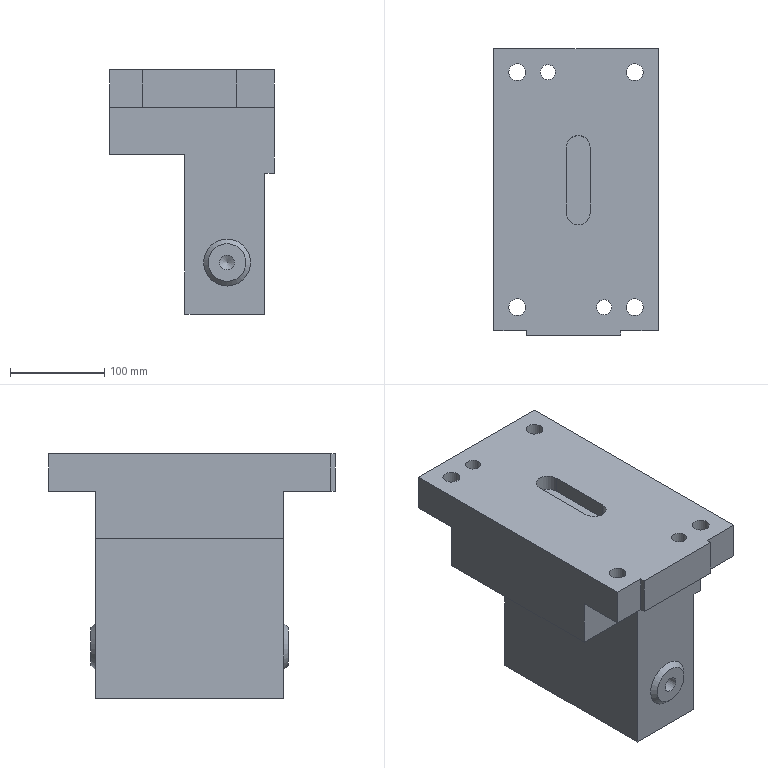Part | NX | features solid 2 | 1 solid | 45 faces | box 175 x 305 x 260 mm | volume 6693790 mm3 | plane 27 | cylinder 14 | cone 4 | commonest cylinder face diameters 16 x4 18 x4 26 x4 25 x2
STEP:
#1=CARTESIAN_POINT('',(856.828,220.,-355.));
#2=VERTEX_POINT('',#1);
#3=CARTESIAN_POINT('',(864.828,220.,-355.));
#4=DIRECTION('',(0.,1.,0.));
#5=DIRECTION('',(-1.,0.,0.));
#6=AXIS2_PLACEMENT_3D('',#3,#4,#5);
#7=CIRCLE('',#6,8.);
#8=EDGE_CURVE('',#2,#2,#7,.T.);
#9=ORIENTED_EDGE('',*,*,#8,.F.);
#10=EDGE_LOOP('',(#9));
#11=FACE_BOUND('',#10,.T.);
#12=CARTESIAN_POINT('',(864.828,224.807,-355.));
#13=VERTEX_POINT('',#12);
#14=VERTEX_LOOP('',#13);
#15=FACE_BOUND('',#14,.T.);
#16=CARTESIAN_POINT('',(864.828,220.,-355.));
#17=DIRECTION('',(0.,-1.,0.));
#18=DIRECTION('',(1.,0.,0.));
#19=AXIS2_PLACEMENT_3D('',#16,#17,#18);
#20=CONICAL_SURFACE('',#19,8.,1.03);
#21=ADVANCED_FACE('',(#11,#15),#20,.F.);
#22=ORIENTED_EDGE('',*,*,#8,.T.);
#23=EDGE_LOOP('',(#22));
#24=FACE_BOUND('',#23,.T.);
#25=CARTESIAN_POINT('',(856.828,195.,-355.));
#26=VERTEX_POINT('',#25);
#27=CARTESIAN_POINT('',(864.828,195.,-355.));
#28=DIRECTION('',(0.,1.,0.));
#29=DIRECTION('',(-1.,0.,0.));
#30=AXIS2_PLACEMENT_3D('',#27,#28,#29);
#31=CIRCLE('',#30,8.);
#32=EDGE_CURVE('',#26,#26,#31,.T.);
#33=ORIENTED_EDGE('',*,*,#32,.F.);
#34=EDGE_LOOP('',(#33));
#35=FACE_BOUND('',#34,.T.);
#36=CARTESIAN_POINT('',(864.828,160.,-355.));
#37=DIRECTION('',(0.,1.,0.));
#38=DIRECTION('',(-1.,0.,0.));
#39=AXIS2_PLACEMENT_3D('',#36,#37,#38);
#40=CYLINDRICAL_SURFACE('',#39,8.);
#41=ADVANCED_FACE('',(#24,#35),#40,.F.);
#42=ORIENTED_EDGE('',*,*,#32,.T.);
#43=EDGE_LOOP('',(#42));
#44=FACE_BOUND('',#43,.T.);
#45=CARTESIAN_POINT('',(864.828,195.,-335.));
#46=VERTEX_POINT('',#45);
#47=CARTESIAN_POINT('',(864.828,195.,-355.));
#48=DIRECTION('',(0.,-1.,0.));
#49=DIRECTION('',(0.,0.,1.));
#50=AXIS2_PLACEMENT_3D('',#47,#48,#49);
#51=CIRCLE('',#50,20.);
#52=EDGE_CURVE('',#46,#46,#51,.F.);
#53=ORIENTED_EDGE('',*,*,#52,.F.);
#54=EDGE_LOOP('',(#53));
#55=FACE_BOUND('',#54,.T.);
#56=CARTESIAN_POINT('',(889.828,195.,-380.));
#57=DIRECTION('',(0.,1.,0.));
#58=DIRECTION('',(-1.,0.,0.));
#59=AXIS2_PLACEMENT_3D('',#56,#57,#58);
#60=PLANE('',#59);
#61=ADVANCED_FACE('',(#44,#55),#60,.F.);
#62=CARTESIAN_POINT('',(756.,175.,-175.));
#63=VERTEX_POINT('',#62);
#64=CARTESIAN_POINT('',(765.,175.,-175.));
#65=DIRECTION('',(0.,0.,1.));
#66=DIRECTION('',(-1.,0.,0.));
#67=AXIS2_PLACEMENT_3D('',#64,#65,#66);
#68=CIRCLE('',#67,9.);
#69=EDGE_CURVE('',#63,#63,#68,.F.);
#70=ORIENTED_EDGE('',*,*,#69,.F.);
#71=EDGE_LOOP('',(#70));
#72=FACE_BOUND('',#71,.T.);
#73=CARTESIAN_POINT('',(752.,175.,-175.));
#74=VERTEX_POINT('',#73);
#75=CARTESIAN_POINT('',(765.,175.,-175.));
#76=DIRECTION('',(0.,0.,1.));
#77=DIRECTION('',(-1.,0.,0.));
#78=AXIS2_PLACEMENT_3D('',#75,#76,#77);
#79=CIRCLE('',#78,13.);
#80=EDGE_CURVE('',#74,#74,#79,.T.);
#81=ORIENTED_EDGE('',*,*,#80,.F.);
#82=EDGE_LOOP('',(#81));
#83=FACE_BOUND('',#82,.T.);
#84=CARTESIAN_POINT('',(765.,155.,-175.));
#85=DIRECTION('',(0.,0.,1.));
#86=DIRECTION('',(0.,1.,0.));
#87=AXIS2_PLACEMENT_3D('',#84,#85,#86);
#88=PLANE('',#87);
#89=ADVANCED_FACE('',(#72,#83),#88,.F.);
#90=CARTESIAN_POINT('',(881.,175.,-175.));
#91=VERTEX_POINT('',#90);
#92=CARTESIAN_POINT('',(890.,175.,-175.));
#93=DIRECTION('',(0.,0.,1.));
#94=DIRECTION('',(-1.,0.,0.));
#95=AXIS2_PLACEMENT_3D('',#92,#93,#94);
#96=CIRCLE('',#95,9.);
#97=EDGE_CURVE('',#91,#91,#96,.F.);
#98=ORIENTED_EDGE('',*,*,#97,.F.);
#99=EDGE_LOOP('',(#98));
#100=FACE_BOUND('',#99,.T.);
#101=CARTESIAN_POINT('',(877.,175.,-175.));
#102=VERTEX_POINT('',#101);
#103=CARTESIAN_POINT('',(890.,175.,-175.));
#104=DIRECTION('',(0.,0.,1.));
#105=DIRECTION('',(-1.,0.,0.));
#106=AXIS2_PLACEMENT_3D('',#103,#104,#105);
#107=CIRCLE('',#106,13.);
#108=EDGE_CURVE('',#102,#102,#107,.T.);
#109=ORIENTED_EDGE('',*,*,#108,.F.);
#110=EDGE_LOOP('',(#109));
#111=FACE_BOUND('',#110,.T.);
#112=CARTESIAN_POINT('',(890.,155.,-175.));
#113=DIRECTION('',(0.,0.,1.));
#114=DIRECTION('',(0.,1.,0.));
#115=AXIS2_PLACEMENT_3D('',#112,#113,#114);
#116=PLANE('',#115);
#117=ADVANCED_FACE('',(#100,#111),#116,.F.);
#118=CARTESIAN_POINT('',(864.828,200.,-330.));
#119=VERTEX_POINT('',#118);
#120=CARTESIAN_POINT('',(864.828,200.,-355.));
#121=DIRECTION('',(0.,1.,0.));
#122=DIRECTION('',(0.,0.,1.));
#123=AXIS2_PLACEMENT_3D('',#120,#121,#122);
#124=CIRCLE('',#123,25.);
#125=EDGE_CURVE('',#119,#119,#124,.T.);
#126=ORIENTED_EDGE('',*,*,#125,.F.);
#127=EDGE_LOOP('',(#126));
#128=FACE_BOUND('',#127,.T.);
#129=ORIENTED_EDGE('',*,*,#52,.T.);
#130=EDGE_LOOP('',(#129));
#131=FACE_BOUND('',#130,.T.);
#132=CARTESIAN_POINT('',(864.828,195.,-355.));
#133=DIRECTION('',(0.,1.,0.));
#134=DIRECTION('',(0.,0.,1.));
#135=AXIS2_PLACEMENT_3D('',#132,#133,#134);
#136=CONICAL_SURFACE('',#135,20.,0.7854);
#137=ADVANCED_FACE('',(#128,#131),#136,.T.);
#138=ORIENTED_EDGE('',*,*,#80,.T.);
#139=EDGE_LOOP('',(#138));
#140=FACE_BOUND('',#139,.T.);
#141=CARTESIAN_POINT('',(752.,175.,-190.));
#142=VERTEX_POINT('',#141);
#143=CARTESIAN_POINT('',(765.,175.,-190.));
#144=DIRECTION('',(0.,0.,1.));
#145=DIRECTION('',(-1.,0.,0.));
#146=AXIS2_PLACEMENT_3D('',#143,#144,#145);
#147=CIRCLE('',#146,13.);
#148=EDGE_CURVE('',#142,#142,#147,.F.);
#149=ORIENTED_EDGE('',*,*,#148,.T.);
#150=EDGE_LOOP('',(#149));
#151=FACE_BOUND('',#150,.T.);
#152=CARTESIAN_POINT('',(765.,175.,-235.));
#153=DIRECTION('',(0.,0.,-1.));
#154=DIRECTION('',(0.,-1.,0.));
#155=AXIS2_PLACEMENT_3D('',#152,#153,#154);
#156=CYLINDRICAL_SURFACE('',#155,13.);
#157=ADVANCED_FACE('',(#140,#151),#156,.F.);
#158=ORIENTED_EDGE('',*,*,#108,.T.);
#159=EDGE_LOOP('',(#158));
#160=FACE_BOUND('',#159,.T.);
#161=CARTESIAN_POINT('',(877.,175.,-190.));
#162=VERTEX_POINT('',#161);
#163=CARTESIAN_POINT('',(890.,175.,-190.));
#164=DIRECTION('',(0.,0.,1.));
#165=DIRECTION('',(-1.,0.,0.));
#166=AXIS2_PLACEMENT_3D('',#163,#164,#165);
#167=CIRCLE('',#166,13.);
#168=EDGE_CURVE('',#162,#162,#167,.F.);
#169=ORIENTED_EDGE('',*,*,#168,.T.);
#170=EDGE_LOOP('',(#169));
#171=FACE_BOUND('',#170,.T.);
#172=CARTESIAN_POINT('',(890.,175.,-235.));
#173=DIRECTION('',(0.,0.,-1.));
#174=DIRECTION('',(0.,-1.,0.));
#175=AXIS2_PLACEMENT_3D('',#172,#173,#174);
#176=CYLINDRICAL_SURFACE('',#175,13.);
#177=ADVANCED_FACE('',(#160,#171),#176,.F.);
#178=CARTESIAN_POINT('',(875.,150.,-150.));
#179=VERTEX_POINT('',#178);
#180=CARTESIAN_POINT('',(875.,150.,-190.));
#181=VERTEX_POINT('',#180);
#182=CARTESIAN_POINT('',(875.,150.,-140.));
#183=DIRECTION('',(0.,0.,-1.));
#184=VECTOR('',#183,1000.);
#185=LINE('',#182,#184);
#186=EDGE_CURVE('',#179,#181,#185,.T.);
#187=ORIENTED_EDGE('',*,*,#186,.F.);
#188=CARTESIAN_POINT('',(875.,145.,-150.));
#189=VERTEX_POINT('',#188);
#190=CARTESIAN_POINT('',(875.,80.,-150.));
#191=DIRECTION('',(0.,-1.,0.));
#192=VECTOR('',#191,1000.);
#193=LINE('',#190,#192);
#194=EDGE_CURVE('',#179,#189,#193,.T.);
#195=ORIENTED_EDGE('',*,*,#194,.T.);
#196=CARTESIAN_POINT('',(875.,145.,-190.));
#197=VERTEX_POINT('',#196);
#198=CARTESIAN_POINT('',(875.,145.,-140.));
#199=DIRECTION('',(0.,0.,-1.));
#200=VECTOR('',#199,1000.);
#201=LINE('',#198,#200);
#202=EDGE_CURVE('',#189,#197,#201,.T.);
#203=ORIENTED_EDGE('',*,*,#202,.T.);
#204=CARTESIAN_POINT('',(875.,80.,-190.));
#205=DIRECTION('',(0.,1.,0.));
#206=VECTOR('',#205,1000.);
#207=LINE('',#204,#206);
#208=EDGE_CURVE('',#197,#181,#207,.T.);
#209=ORIENTED_EDGE('',*,*,#208,.T.);
#210=EDGE_LOOP('',(#187,#195,#203,#209));
#211=FACE_BOUND('',#210,.T.);
#212=CARTESIAN_POINT('',(875.,80.,-140.));
#213=DIRECTION('',(1.,0.,0.));
#214=DIRECTION('',(0.,0.,1.));
#215=AXIS2_PLACEMENT_3D('',#212,#213,#214);
#216=PLANE('',#215);
#217=ADVANCED_FACE('',(#211),#216,.T.);
#218=ORIENTED_EDGE('',*,*,#202,.F.);
#219=CARTESIAN_POINT('',(775.,145.,-150.));
#220=VERTEX_POINT('',#219);
#221=CARTESIAN_POINT('',(827.5,145.,-150.));
#222=DIRECTION('',(-1.,0.,0.));
#223=VECTOR('',#222,1000.);
#224=LINE('',#221,#223);
#225=EDGE_CURVE('',#189,#220,#224,.T.);
#226=ORIENTED_EDGE('',*,*,#225,.T.);
#227=CARTESIAN_POINT('',(775.,145.,-190.));
#228=VERTEX_POINT('',#227);
#229=CARTESIAN_POINT('',(775.,145.,-140.));
#230=DIRECTION('',(0.,0.,1.));
#231=VECTOR('',#230,1000.);
#232=LINE('',#229,#231);
#233=EDGE_CURVE('',#228,#220,#232,.T.);
#234=ORIENTED_EDGE('',*,*,#233,.F.);
#235=CARTESIAN_POINT('',(665.,145.,-190.));
#236=DIRECTION('',(1.,0.,0.));
#237=VECTOR('',#236,1000.);
#238=LINE('',#235,#237);
#239=EDGE_CURVE('',#228,#197,#238,.T.);
#240=ORIENTED_EDGE('',*,*,#239,.T.);
#241=EDGE_LOOP('',(#218,#226,#234,#240));
#242=FACE_BOUND('',#241,.T.);
#243=CARTESIAN_POINT('',(827.5,145.,-170.));
#244=DIRECTION('',(0.,-1.,0.));
#245=DIRECTION('',(0.,0.,1.));
#246=AXIS2_PLACEMENT_3D('',#243,#244,#245);
#247=PLANE('',#246);
#248=ADVANCED_FACE('',(#242),#247,.T.);
#249=ORIENTED_EDGE('',*,*,#233,.T.);
#250=CARTESIAN_POINT('',(775.,150.,-150.));
#251=VERTEX_POINT('',#250);
#252=CARTESIAN_POINT('',(775.,80.,-150.));
#253=DIRECTION('',(0.,1.,0.));
#254=VECTOR('',#253,1000.);
#255=LINE('',#252,#254);
#256=EDGE_CURVE('',#220,#251,#255,.T.);
#257=ORIENTED_EDGE('',*,*,#256,.T.);
#258=CARTESIAN_POINT('',(775.,150.,-190.));
#259=VERTEX_POINT('',#258);
#260=CARTESIAN_POINT('',(775.,150.,-140.));
#261=DIRECTION('',(0.,0.,1.));
#262=VECTOR('',#261,1000.);
#263=LINE('',#260,#262);
#264=EDGE_CURVE('',#259,#251,#263,.T.);
#265=ORIENTED_EDGE('',*,*,#264,.F.);
#266=CARTESIAN_POINT('',(775.,80.,-190.));
#267=DIRECTION('',(0.,1.,0.));
#268=VECTOR('',#267,1000.);
#269=LINE('',#266,#268);
#270=EDGE_CURVE('',#228,#259,#269,.T.);
#271=ORIENTED_EDGE('',*,*,#270,.F.);
#272=EDGE_LOOP('',(#249,#257,#265,#271));
#273=FACE_BOUND('',#272,.T.);
#274=CARTESIAN_POINT('',(775.,80.,-140.));
#275=DIRECTION('',(-1.,0.,0.));
#276=DIRECTION('',(0.,0.,-1.));
#277=AXIS2_PLACEMENT_3D('',#274,#275,#276);
#278=PLANE('',#277);
#279=ADVANCED_FACE('',(#273),#278,.T.);
#280=ORIENTED_EDGE('',*,*,#69,.T.);
#281=EDGE_LOOP('',(#280));
#282=FACE_BOUND('',#281,.T.);
#283=CARTESIAN_POINT('',(774.,175.,-150.));
#284=VERTEX_POINT('',#283);
#285=CARTESIAN_POINT('',(765.,175.,-150.));
#286=DIRECTION('',(0.,0.,-1.));
#287=DIRECTION('',(1.,0.,0.));
#288=AXIS2_PLACEMENT_3D('',#285,#286,#287);
#289=CIRCLE('',#288,9.);
#290=EDGE_CURVE('',#284,#284,#289,.F.);
#291=ORIENTED_EDGE('',*,*,#290,.T.);
#292=EDGE_LOOP('',(#291));
#293=FACE_BOUND('',#292,.T.);
#294=CARTESIAN_POINT('',(765.,175.,-235.));
#295=DIRECTION('',(0.,0.,1.));
#296=DIRECTION('',(0.,1.,0.));
#297=AXIS2_PLACEMENT_3D('',#294,#295,#296);
#298=CYLINDRICAL_SURFACE('',#297,9.);
#299=ADVANCED_FACE('',(#282,#293),#298,.F.);
#300=ORIENTED_EDGE('',*,*,#97,.T.);
#301=EDGE_LOOP('',(#300));
#302=FACE_BOUND('',#301,.T.);
#303=CARTESIAN_POINT('',(899.,175.,-150.));
#304=VERTEX_POINT('',#303);
#305=CARTESIAN_POINT('',(890.,175.,-150.));
#306=DIRECTION('',(0.,0.,-1.));
#307=DIRECTION('',(1.,0.,0.));
#308=AXIS2_PLACEMENT_3D('',#305,#306,#307);
#309=CIRCLE('',#308,9.);
#310=EDGE_CURVE('',#304,#304,#309,.F.);
#311=ORIENTED_EDGE('',*,*,#310,.T.);
#312=EDGE_LOOP('',(#311));
#313=FACE_BOUND('',#312,.T.);
#314=CARTESIAN_POINT('',(890.,175.,-235.));
#315=DIRECTION('',(0.,0.,1.));
#316=DIRECTION('',(0.,1.,0.));
#317=AXIS2_PLACEMENT_3D('',#314,#315,#316);
#318=CYLINDRICAL_SURFACE('',#317,9.);
#319=ADVANCED_FACE('',(#302,#313),#318,.F.);
#320=CARTESIAN_POINT('',(849.5,175.,-190.));
#321=VERTEX_POINT('',#320);
#322=CARTESIAN_POINT('',(857.5,175.,-190.));
#323=DIRECTION('',(0.,0.,1.));
#324=DIRECTION('',(-1.,0.,0.));
#325=AXIS2_PLACEMENT_3D('',#322,#323,#324);
#326=CIRCLE('',#325,8.);
#327=EDGE_CURVE('',#321,#321,#326,.F.);
#328=ORIENTED_EDGE('',*,*,#327,.T.);
#329=EDGE_LOOP('',(#328));
#330=FACE_BOUND('',#329,.T.);
#331=CARTESIAN_POINT('',(865.5,175.,-150.));
#332=VERTEX_POINT('',#331);
#333=CARTESIAN_POINT('',(857.5,175.,-150.));
#334=DIRECTION('',(0.,0.,-1.));
#335=DIRECTION('',(1.,0.,0.));
#336=AXIS2_PLACEMENT_3D('',#333,#334,#335);
#337=CIRCLE('',#336,8.);
#338=EDGE_CURVE('',#332,#332,#337,.F.);
#339=ORIENTED_EDGE('',*,*,#338,.T.);
#340=EDGE_LOOP('',(#339));
#341=FACE_BOUND('',#340,.T.);
#342=CARTESIAN_POINT('',(857.5,175.,-200.));
#343=DIRECTION('',(0.,0.,-1.));
#344=DIRECTION('',(0.,1.,0.));
#345=AXIS2_PLACEMENT_3D('',#342,#343,#344);
#346=CYLINDRICAL_SURFACE('',#345,8.);
#347=ADVANCED_FACE('',(#330,#341),#346,.F.);
#348=CARTESIAN_POINT('',(740.,150.,-190.));
#349=VERTEX_POINT('',#348);
#350=CARTESIAN_POINT('',(665.,150.,-190.));
#351=DIRECTION('',(1.,0.,0.));
#352=VECTOR('',#351,1000.);
#353=LINE('',#350,#352);
#354=EDGE_CURVE('',#349,#259,#353,.T.);
#355=ORIENTED_EDGE('',*,*,#354,.T.);
#356=ORIENTED_EDGE('',*,*,#264,.T.);
#357=CARTESIAN_POINT('',(740.,150.,-150.));
#358=VERTEX_POINT('',#357);
#359=CARTESIAN_POINT('',(575.,150.,-150.));
#360=DIRECTION('',(1.,0.,0.));
#361=VECTOR('',#360,1000.);
#362=LINE('',#359,#361);
#363=EDGE_CURVE('',#358,#251,#362,.T.);
#364=ORIENTED_EDGE('',*,*,#363,.F.);
#365=CARTESIAN_POINT('',(740.,150.,-150.));
#366=DIRECTION('',(0.,0.,-1.));
#367=VECTOR('',#366,1000.);
#368=LINE('',#365,#367);
#369=EDGE_CURVE('',#349,#358,#368,.F.);
#370=ORIENTED_EDGE('',*,*,#369,.F.);
#371=EDGE_LOOP('',(#355,#356,#364,#370));
#372=FACE_BOUND('',#371,.T.);
#373=CARTESIAN_POINT('',(665.,150.,-150.));
#374=DIRECTION('',(0.,1.,0.));
#375=DIRECTION('',(0.,0.,-1.));
#376=AXIS2_PLACEMENT_3D('',#373,#374,#375);
#377=PLANE('',#376);
#378=ADVANCED_FACE('',(#372),#377,.F.);
#379=ORIENTED_EDGE('',*,*,#125,.T.);
#380=EDGE_LOOP('',(#379));
#381=FACE_BOUND('',#380,.T.);
#382=CARTESIAN_POINT('',(740.,200.,-240.));
#383=VERTEX_POINT('',#382);
#384=CARTESIAN_POINT('',(740.,200.,-190.));
#385=VERTEX_POINT('',#384);
#386=CARTESIAN_POINT('',(740.,200.,-435.));
#387=DIRECTION('',(0.,0.,-1.));
#388=VECTOR('',#387,1000.);
#389=LINE('',#386,#388);
#390=EDGE_CURVE('',#383,#385,#389,.F.);
#391=ORIENTED_EDGE('',*,*,#390,.F.);
#392=CARTESIAN_POINT('',(820.,200.,-240.));
#393=VERTEX_POINT('',#392);
#394=CARTESIAN_POINT('',(740.,200.,-240.));
#395=DIRECTION('',(1.,0.,0.));
#396=VECTOR('',#395,1000.);
#397=LINE('',#394,#396);
#398=EDGE_CURVE('',#383,#393,#397,.T.);
#399=ORIENTED_EDGE('',*,*,#398,.T.);
#400=CARTESIAN_POINT('',(820.,200.,-410.));
#401=VERTEX_POINT('',#400);
#402=CARTESIAN_POINT('',(820.,200.,-750.));
#403=DIRECTION('',(0.,0.,-1.));
#404=VECTOR('',#403,1000.);
#405=LINE('',#402,#404);
#406=EDGE_CURVE('',#393,#401,#405,.T.);
#407=ORIENTED_EDGE('',*,*,#406,.T.);
#408=CARTESIAN_POINT('',(905.,200.,-410.));
#409=VERTEX_POINT('',#408);
#410=CARTESIAN_POINT('',(790.,200.,-410.));
#411=DIRECTION('',(-1.,0.,0.));
#412=VECTOR('',#411,1000.);
#413=LINE('',#410,#412);
#414=EDGE_CURVE('',#409,#401,#413,.T.);
#415=ORIENTED_EDGE('',*,*,#414,.F.);
#416=CARTESIAN_POINT('',(905.,200.,-260.));
#417=VERTEX_POINT('',#416);
#418=CARTESIAN_POINT('',(905.,200.,-370.));
#419=DIRECTION('',(0.,0.,1.));
#420=VECTOR('',#419,1000.);
#421=LINE('',#418,#420);
#422=EDGE_CURVE('',#409,#417,#421,.T.);
#423=ORIENTED_EDGE('',*,*,#422,.T.);
#424=CARTESIAN_POINT('',(915.,200.,-260.));
#425=VERTEX_POINT('',#424);
#426=CARTESIAN_POINT('',(915.,200.,-260.));
#427=DIRECTION('',(1.,0.,0.));
#428=VECTOR('',#427,1000.);
#429=LINE('',#426,#428);
#430=EDGE_CURVE('',#417,#425,#429,.T.);
#431=ORIENTED_EDGE('',*,*,#430,.T.);
#432=CARTESIAN_POINT('',(915.,200.,-190.));
#433=VERTEX_POINT('',#432);
#434=CARTESIAN_POINT('',(915.,200.,-225.));
#435=DIRECTION('',(0.,0.,1.));
#436=VECTOR('',#435,1000.);
#437=LINE('',#434,#436);
#438=EDGE_CURVE('',#433,#425,#437,.F.);
#439=ORIENTED_EDGE('',*,*,#438,.F.);
#440=CARTESIAN_POINT('',(760.357,200.,-190.));
#441=DIRECTION('',(1.,0.,0.));
#442=VECTOR('',#441,1000.);
#443=LINE('',#440,#442);
#444=EDGE_CURVE('',#385,#433,#443,.T.);
#445=ORIENTED_EDGE('',*,*,#444,.F.);
#446=EDGE_LOOP('',(#391,#399,#407,#415,#423,#431,#439,#445));
#447=FACE_BOUND('',#446,.T.);
#448=CARTESIAN_POINT('',(820.,200.,-407.));
#449=DIRECTION('',(0.,-1.,0.));
#450=DIRECTION('',(0.,0.,1.));
#451=AXIS2_PLACEMENT_3D('',#448,#449,#450);
#452=PLANE('',#451);
#453=ADVANCED_FACE('',(#381,#447),#452,.T.);
#454=ORIENTED_EDGE('',*,*,#327,.F.);
#455=EDGE_LOOP('',(#454));
#456=FACE_BOUND('',#455,.T.);
#457=ORIENTED_EDGE('',*,*,#168,.F.);
#458=EDGE_LOOP('',(#457));
#459=FACE_BOUND('',#458,.T.);
#460=ORIENTED_EDGE('',*,*,#148,.F.);
#461=EDGE_LOOP('',(#460));
#462=FACE_BOUND('',#461,.T.);
#463=CARTESIAN_POINT('',(740.,-295.,-190.));
#464=DIRECTION('',(0.,-1.,0.));
#465=VECTOR('',#464,1000.);
#466=LINE('',#463,#465);
#467=EDGE_CURVE('',#349,#385,#466,.F.);
#468=ORIENTED_EDGE('',*,*,#467,.T.);
#469=ORIENTED_EDGE('',*,*,#444,.T.);
#470=CARTESIAN_POINT('',(915.,150.,-190.));
#471=VERTEX_POINT('',#470);
#472=CARTESIAN_POINT('',(915.,-295.,-190.));
#473=DIRECTION('',(0.,1.,0.));
#474=VECTOR('',#473,1000.);
#475=LINE('',#472,#474);
#476=EDGE_CURVE('',#433,#471,#475,.F.);
#477=ORIENTED_EDGE('',*,*,#476,.T.);
#478=CARTESIAN_POINT('',(665.,150.,-190.));
#479=DIRECTION('',(1.,0.,0.));
#480=VECTOR('',#479,1000.);
#481=LINE('',#478,#480);
#482=EDGE_CURVE('',#181,#471,#481,.T.);
#483=ORIENTED_EDGE('',*,*,#482,.F.);
#484=ORIENTED_EDGE('',*,*,#208,.F.);
#485=ORIENTED_EDGE('',*,*,#239,.F.);
#486=ORIENTED_EDGE('',*,*,#270,.T.);
#487=ORIENTED_EDGE('',*,*,#354,.F.);
#488=EDGE_LOOP('',(#468,#469,#477,#483,#484,#485,#486,#487));
#489=FACE_BOUND('',#488,.T.);
#490=CARTESIAN_POINT('',(655.,-295.,-190.));
#491=DIRECTION('',(0.,0.,1.));
#492=DIRECTION('',(1.,0.,0.));
#493=AXIS2_PLACEMENT_3D('',#490,#491,#492);
#494=PLANE('',#493);
#495=ADVANCED_FACE('',(#456,#459,#462,#489),#494,.F.);
#496=CARTESIAN_POINT('',(915.,150.,-150.));
#497=VERTEX_POINT('',#496);
#498=CARTESIAN_POINT('',(575.,150.,-150.));
#499=DIRECTION('',(1.,0.,0.));
#500=VECTOR('',#499,1000.);
#501=LINE('',#498,#500);
#502=EDGE_CURVE('',#179,#497,#501,.T.);
#503=ORIENTED_EDGE('',*,*,#502,.F.);
#504=ORIENTED_EDGE('',*,*,#186,.T.);
#505=ORIENTED_EDGE('',*,*,#482,.T.);
#506=CARTESIAN_POINT('',(915.,150.,-150.));
#507=DIRECTION('',(0.,0.,1.));
#508=VECTOR('',#507,1000.);
#509=LINE('',#506,#508);
#510=EDGE_CURVE('',#497,#471,#509,.F.);
#511=ORIENTED_EDGE('',*,*,#510,.F.);
#512=EDGE_LOOP('',(#503,#504,#505,#511));
#513=FACE_BOUND('',#512,.T.);
#514=CARTESIAN_POINT('',(665.,150.,-150.));
#515=DIRECTION('',(0.,1.,0.));
#516=DIRECTION('',(0.,0.,-1.));
#517=AXIS2_PLACEMENT_3D('',#514,#515,#516);
#518=PLANE('',#517);
#519=ADVANCED_FACE('',(#513),#518,.F.);
#520=CARTESIAN_POINT('',(915.,400.,-260.));
#521=VERTEX_POINT('',#520);
#522=CARTESIAN_POINT('',(915.,325.,-260.));
#523=DIRECTION('',(0.,-1.,0.));
#524=VECTOR('',#523,1000.);
#525=LINE('',#522,#524);
#526=EDGE_CURVE('',#425,#521,#525,.F.);
#527=ORIENTED_EDGE('',*,*,#526,.T.);
#528=CARTESIAN_POINT('',(915.,400.,-190.));
#529=VERTEX_POINT('',#528);
#530=CARTESIAN_POINT('',(915.,400.,-167.143));
#531=DIRECTION('',(0.,0.,1.));
#532=VECTOR('',#531,1000.);
#533=LINE('',#530,#532);
#534=EDGE_CURVE('',#521,#529,#533,.T.);
#535=ORIENTED_EDGE('',*,*,#534,.T.);
#536=CARTESIAN_POINT('',(915.,450.,-190.));
#537=VERTEX_POINT('',#536);
#538=CARTESIAN_POINT('',(915.,300.,-190.));
#539=DIRECTION('',(0.,1.,0.));
#540=VECTOR('',#539,1000.);
#541=LINE('',#538,#540);
#542=EDGE_CURVE('',#529,#537,#541,.T.);
#543=ORIENTED_EDGE('',*,*,#542,.T.);
#544=CARTESIAN_POINT('',(915.,450.,-150.));
#545=VERTEX_POINT('',#544);
#546=CARTESIAN_POINT('',(915.,450.,-150.));
#547=DIRECTION('',(0.,0.,1.));
#548=VECTOR('',#547,1000.);
#549=LINE('',#546,#548);
#550=EDGE_CURVE('',#545,#537,#549,.F.);
#551=ORIENTED_EDGE('',*,*,#550,.F.);
#552=CARTESIAN_POINT('',(915.,340.,-150.));
#553=DIRECTION('',(0.,-1.,0.));
#554=VECTOR('',#553,1000.);
#555=LINE('',#552,#554);
#556=EDGE_CURVE('',#497,#545,#555,.F.);
#557=ORIENTED_EDGE('',*,*,#556,.F.);
#558=ORIENTED_EDGE('',*,*,#510,.T.);
#559=ORIENTED_EDGE('',*,*,#476,.F.);
#560=ORIENTED_EDGE('',*,*,#438,.T.);
#561=EDGE_LOOP('',(#527,#535,#543,#551,#557,#558,#559,#560));
#562=FACE_BOUND('',#561,.T.);
#563=CARTESIAN_POINT('',(915.,250.,-225.));
#564=DIRECTION('',(1.,0.,0.));
#565=DIRECTION('',(0.,0.,-1.));
#566=AXIS2_PLACEMENT_3D('',#563,#564,#565);
#567=PLANE('',#566);
#568=ADVANCED_FACE('',(#562),#567,.T.);
#569=CARTESIAN_POINT('',(740.,450.,-150.));
#570=VERTEX_POINT('',#569);
#571=CARTESIAN_POINT('',(740.,175.,-150.));
#572=DIRECTION('',(0.,-1.,0.));
#573=VECTOR('',#572,1000.);
#574=LINE('',#571,#573);
#575=EDGE_CURVE('',#570,#358,#574,.T.);
#576=ORIENTED_EDGE('',*,*,#575,.F.);
#577=CARTESIAN_POINT('',(740.,450.,-190.));
#578=VERTEX_POINT('',#577);
#579=CARTESIAN_POINT('',(740.,450.,-150.));
#580=DIRECTION('',(0.,0.,-1.));
#581=VECTOR('',#580,1000.);
#582=LINE('',#579,#581);
#583=EDGE_CURVE('',#578,#570,#582,.F.);
#584=ORIENTED_EDGE('',*,*,#583,.F.);
#585=CARTESIAN_POINT('',(740.,400.,-190.));
#586=VERTEX_POINT('',#585);
#587=CARTESIAN_POINT('',(740.,225.,-190.));
#588=DIRECTION('',(0.,-1.,0.));
#589=VECTOR('',#588,1000.);
#590=LINE('',#587,#589);
#591=EDGE_CURVE('',#578,#586,#590,.T.);
#592=ORIENTED_EDGE('',*,*,#591,.T.);
#593=CARTESIAN_POINT('',(740.,400.,-240.));
#594=VERTEX_POINT('',#593);
#595=CARTESIAN_POINT('',(740.,400.,-167.143));
#596=DIRECTION('',(0.,0.,-1.));
#597=VECTOR('',#596,1000.);
#598=LINE('',#595,#597);
#599=EDGE_CURVE('',#594,#586,#598,.F.);
#600=ORIENTED_EDGE('',*,*,#599,.F.);
#601=CARTESIAN_POINT('',(740.,175.,-240.));
#602=DIRECTION('',(0.,-1.,0.));
#603=VECTOR('',#602,1000.);
#604=LINE('',#601,#603);
#605=EDGE_CURVE('',#383,#594,#604,.F.);
#606=ORIENTED_EDGE('',*,*,#605,.F.);
#607=ORIENTED_EDGE('',*,*,#390,.T.);
#608=ORIENTED_EDGE('',*,*,#467,.F.);
#609=ORIENTED_EDGE('',*,*,#369,.T.);
#610=EDGE_LOOP('',(#576,#584,#592,#600,#606,#607,#608,#609));
#611=FACE_BOUND('',#610,.T.);
#612=CARTESIAN_POINT('',(740.,175.,-435.));
#613=DIRECTION('',(-1.,0.,0.));
#614=DIRECTION('',(0.,0.,1.));
#615=AXIS2_PLACEMENT_3D('',#612,#613,#614);
#616=PLANE('',#615);
#617=ADVANCED_FACE('',(#611),#616,.T.);
#618=CARTESIAN_POINT('',(842.5,345.,-150.));
#619=VERTEX_POINT('',#618);
#620=CARTESIAN_POINT('',(842.5,275.,-150.));
#621=VERTEX_POINT('',#620);
#622=CARTESIAN_POINT('',(842.5,325.,-150.));
#623=DIRECTION('',(0.,-1.,0.));
#624=VECTOR('',#623,1000.);
#625=LINE('',#622,#624);
#626=EDGE_CURVE('',#619,#621,#625,.T.);
#627=ORIENTED_EDGE('',*,*,#626,.T.);
#628=CARTESIAN_POINT('',(817.5,275.,-150.));
#629=VERTEX_POINT('',#628);
#630=CARTESIAN_POINT('',(830.,275.,-150.));
#631=DIRECTION('',(0.,0.,-1.));
#632=DIRECTION('',(-1.,0.,0.));
#633=AXIS2_PLACEMENT_3D('',#630,#631,#632);
#634=CIRCLE('',#633,12.5);
#635=EDGE_CURVE('',#621,#629,#634,.T.);
#636=ORIENTED_EDGE('',*,*,#635,.T.);
#637=CARTESIAN_POINT('',(817.5,345.,-150.));
#638=VERTEX_POINT('',#637);
#639=CARTESIAN_POINT('',(817.5,325.,-150.));
#640=DIRECTION('',(0.,1.,0.));
#641=VECTOR('',#640,1000.);
#642=LINE('',#639,#641);
#643=EDGE_CURVE('',#629,#638,#642,.T.);
#644=ORIENTED_EDGE('',*,*,#643,.T.);
#645=CARTESIAN_POINT('',(830.,345.,-150.));
#646=DIRECTION('',(0.,0.,-1.));
#647=DIRECTION('',(-1.,0.,0.));
#648=AXIS2_PLACEMENT_3D('',#645,#646,#647);
#649=CIRCLE('',#648,12.5);
#650=EDGE_CURVE('',#638,#619,#649,.T.);
#651=ORIENTED_EDGE('',*,*,#650,.T.);
#652=EDGE_LOOP('',(#627,#636,#644,#651));
#653=FACE_BOUND('',#652,.T.);
#654=ORIENTED_EDGE('',*,*,#338,.F.);
#655=EDGE_LOOP('',(#654));
#656=FACE_BOUND('',#655,.T.);
#657=ORIENTED_EDGE('',*,*,#310,.F.);
#658=EDGE_LOOP('',(#657));
#659=FACE_BOUND('',#658,.T.);
#660=ORIENTED_EDGE('',*,*,#290,.F.);
#661=EDGE_LOOP('',(#660));
#662=FACE_BOUND('',#661,.T.);
#663=ORIENTED_EDGE('',*,*,#556,.T.);
#664=CARTESIAN_POINT('',(575.,450.,-150.));
#665=DIRECTION('',(1.,0.,0.));
#666=VECTOR('',#665,1000.);
#667=LINE('',#664,#666);
#668=EDGE_CURVE('',#570,#545,#667,.T.);
#669=ORIENTED_EDGE('',*,*,#668,.F.);
#670=ORIENTED_EDGE('',*,*,#575,.T.);
#671=ORIENTED_EDGE('',*,*,#363,.T.);
#672=ORIENTED_EDGE('',*,*,#256,.F.);
#673=ORIENTED_EDGE('',*,*,#225,.F.);
#674=ORIENTED_EDGE('',*,*,#194,.F.);
#675=ORIENTED_EDGE('',*,*,#502,.T.);
#676=EDGE_LOOP('',(#663,#669,#670,#671,#672,#673,#674,#675));
#677=FACE_BOUND('',#676,.T.);
#678=CARTESIAN_POINT('',(774.,425.,-150.));
#679=VERTEX_POINT('',#678);
#680=CARTESIAN_POINT('',(765.,425.,-150.));
#681=DIRECTION('',(0.,0.,-1.));
#682=DIRECTION('',(1.,0.,0.));
#683=AXIS2_PLACEMENT_3D('',#680,#681,#682);
#684=CIRCLE('',#683,9.);
#685=EDGE_CURVE('',#679,#679,#684,.F.);
#686=ORIENTED_EDGE('',*,*,#685,.F.);
#687=EDGE_LOOP('',(#686));
#688=FACE_BOUND('',#687,.T.);
#689=CARTESIAN_POINT('',(899.,425.,-150.));
#690=VERTEX_POINT('',#689);
#691=CARTESIAN_POINT('',(890.,425.,-150.));
#692=DIRECTION('',(0.,0.,-1.));
#693=DIRECTION('',(1.,0.,0.));
#694=AXIS2_PLACEMENT_3D('',#691,#692,#693);
#695=CIRCLE('',#694,9.);
#696=EDGE_CURVE('',#690,#690,#695,.F.);
#697=ORIENTED_EDGE('',*,*,#696,.F.);
#698=EDGE_LOOP('',(#697));
#699=FACE_BOUND('',#698,.T.);
#700=CARTESIAN_POINT('',(805.5,425.,-150.));
#701=VERTEX_POINT('',#700);
#702=CARTESIAN_POINT('',(797.5,425.,-150.));
#703=DIRECTION('',(0.,0.,-1.));
#704=DIRECTION('',(1.,0.,0.));
#705=AXIS2_PLACEMENT_3D('',#702,#703,#704);
#706=CIRCLE('',#705,8.);
#707=EDGE_CURVE('',#701,#701,#706,.F.);
#708=ORIENTED_EDGE('',*,*,#707,.F.);
#709=EDGE_LOOP('',(#708));
#710=FACE_BOUND('',#709,.T.);
#711=CARTESIAN_POINT('',(575.,325.,-150.));
#712=DIRECTION('',(0.,0.,-1.));
#713=DIRECTION('',(1.,0.,0.));
#714=AXIS2_PLACEMENT_3D('',#711,#712,#713);
#715=PLANE('',#714);
#716=ADVANCED_FACE('',(#653,#656,#659,#662,#677,#688,#699,#710),#715,.F.);
#717=CARTESIAN_POINT('',(820.,400.,-410.));
#718=VERTEX_POINT('',#717);
#719=CARTESIAN_POINT('',(820.,325.,-410.));
#720=DIRECTION('',(0.,-1.,0.));
#721=VECTOR('',#720,1000.);
#722=LINE('',#719,#721);
#723=EDGE_CURVE('',#718,#401,#722,.T.);
#724=ORIENTED_EDGE('',*,*,#723,.F.);
#725=CARTESIAN_POINT('',(905.,400.,-410.));
#726=VERTEX_POINT('',#725);
#727=CARTESIAN_POINT('',(790.,400.,-410.));
#728=DIRECTION('',(-1.,0.,0.));
#729=VECTOR('',#728,1000.);
#730=LINE('',#727,#729);
#731=EDGE_CURVE('',#726,#718,#730,.T.);
#732=ORIENTED_EDGE('',*,*,#731,.F.);
#733=CARTESIAN_POINT('',(905.,325.,-410.));
#734=DIRECTION('',(0.,1.,0.));
#735=VECTOR('',#734,1000.);
#736=LINE('',#733,#735);
#737=EDGE_CURVE('',#409,#726,#736,.T.);
#738=ORIENTED_EDGE('',*,*,#737,.F.);
#739=ORIENTED_EDGE('',*,*,#414,.T.);
#740=EDGE_LOOP('',(#724,#732,#738,#739));
#741=FACE_BOUND('',#740,.T.);
#742=CARTESIAN_POINT('',(790.,325.,-410.));
#743=DIRECTION('',(0.,0.,1.));
#744=DIRECTION('',(-1.,0.,0.));
#745=AXIS2_PLACEMENT_3D('',#742,#743,#744);
#746=PLANE('',#745);
#747=ADVANCED_FACE('',(#741),#746,.F.);
#748=ORIENTED_EDGE('',*,*,#737,.T.);
#749=CARTESIAN_POINT('',(905.,400.,-260.));
#750=VERTEX_POINT('',#749);
#751=CARTESIAN_POINT('',(905.,400.,-207.143));
#752=DIRECTION('',(0.,0.,1.));
#753=VECTOR('',#752,1000.);
#754=LINE('',#751,#753);
#755=EDGE_CURVE('',#726,#750,#754,.T.);
#756=ORIENTED_EDGE('',*,*,#755,.T.);
#757=CARTESIAN_POINT('',(905.,325.,-260.));
#758=DIRECTION('',(0.,-1.,0.));
#759=VECTOR('',#758,1000.);
#760=LINE('',#757,#759);
#761=EDGE_CURVE('',#750,#417,#760,.T.);
#762=ORIENTED_EDGE('',*,*,#761,.T.);
#763=ORIENTED_EDGE('',*,*,#422,.F.);
#764=EDGE_LOOP('',(#748,#756,#762,#763));
#765=FACE_BOUND('',#764,.T.);
#766=CARTESIAN_POINT('',(905.,250.,-370.));
#767=DIRECTION('',(1.,0.,0.));
#768=DIRECTION('',(0.,0.,-1.));
#769=AXIS2_PLACEMENT_3D('',#766,#767,#768);
#770=PLANE('',#769);
#771=ADVANCED_FACE('',(#765),#770,.T.);
#772=ORIENTED_EDGE('',*,*,#761,.F.);
#773=CARTESIAN_POINT('',(915.,400.,-260.));
#774=DIRECTION('',(1.,0.,0.));
#775=VECTOR('',#774,1000.);
#776=LINE('',#773,#775);
#777=EDGE_CURVE('',#750,#521,#776,.T.);
#778=ORIENTED_EDGE('',*,*,#777,.T.);
#779=ORIENTED_EDGE('',*,*,#526,.F.);
#780=ORIENTED_EDGE('',*,*,#430,.F.);
#781=EDGE_LOOP('',(#772,#778,#779,#780));
#782=FACE_BOUND('',#781,.T.);
#783=CARTESIAN_POINT('',(915.,325.,-260.));
#784=DIRECTION('',(0.,0.,-1.));
#785=DIRECTION('',(0.,1.,0.));
#786=AXIS2_PLACEMENT_3D('',#783,#784,#785);
#787=PLANE('',#786);
#788=ADVANCED_FACE('',(#782),#787,.T.);
#789=ORIENTED_EDGE('',*,*,#605,.T.);
#790=CARTESIAN_POINT('',(820.,400.,-240.));
#791=VERTEX_POINT('',#790);
#792=CARTESIAN_POINT('',(760.357,400.,-240.));
#793=DIRECTION('',(-1.,0.,0.));
#794=VECTOR('',#793,1000.);
#795=LINE('',#792,#794);
#796=EDGE_CURVE('',#791,#594,#795,.T.);
#797=ORIENTED_EDGE('',*,*,#796,.F.);
#798=CARTESIAN_POINT('',(820.,350.,-240.));
#799=DIRECTION('',(0.,-1.,0.));
#800=VECTOR('',#799,1000.);
#801=LINE('',#798,#800);
#802=EDGE_CURVE('',#791,#393,#801,.T.);
#803=ORIENTED_EDGE('',*,*,#802,.T.);
#804=ORIENTED_EDGE('',*,*,#398,.F.);
#805=EDGE_LOOP('',(#789,#797,#803,#804));
#806=FACE_BOUND('',#805,.T.);
#807=CARTESIAN_POINT('',(740.,350.,-240.));
#808=DIRECTION('',(0.,0.,-1.));
#809=DIRECTION('',(0.,-1.,0.));
#810=AXIS2_PLACEMENT_3D('',#807,#808,#809);
#811=PLANE('',#810);
#812=ADVANCED_FACE('',(#806),#811,.T.);
#813=ORIENTED_EDGE('',*,*,#802,.F.);
#814=CARTESIAN_POINT('',(820.,400.,-207.143));
#815=DIRECTION('',(0.,0.,1.));
#816=VECTOR('',#815,1000.);
#817=LINE('',#814,#816);
#818=EDGE_CURVE('',#718,#791,#817,.T.);
#819=ORIENTED_EDGE('',*,*,#818,.F.);
#820=ORIENTED_EDGE('',*,*,#723,.T.);
#821=ORIENTED_EDGE('',*,*,#406,.F.);
#822=EDGE_LOOP('',(#813,#819,#820,#821));
#823=FACE_BOUND('',#822,.T.);
#824=CARTESIAN_POINT('',(820.,350.,-750.));
#825=DIRECTION('',(-1.,0.,0.));
#826=DIRECTION('',(0.,0.,-1.));
#827=AXIS2_PLACEMENT_3D('',#824,#825,#826);
#828=PLANE('',#827);
#829=ADVANCED_FACE('',(#823),#828,.T.);
#830=CARTESIAN_POINT('',(752.,425.,-175.));
#831=VERTEX_POINT('',#830);
#832=CARTESIAN_POINT('',(765.,425.,-175.));
#833=DIRECTION('',(0.,0.,1.));
#834=DIRECTION('',(-1.,0.,0.));
#835=AXIS2_PLACEMENT_3D('',#832,#833,#834);
#836=CIRCLE('',#835,13.);
#837=EDGE_CURVE('',#831,#831,#836,.T.);
#838=ORIENTED_EDGE('',*,*,#837,.T.);
#839=EDGE_LOOP('',(#838));
#840=FACE_BOUND('',#839,.T.);
#841=CARTESIAN_POINT('',(778.,425.,-190.));
#842=VERTEX_POINT('',#841);
#843=CARTESIAN_POINT('',(765.,425.,-190.));
#844=DIRECTION('',(0.,0.,-1.));
#845=DIRECTION('',(1.,0.,0.));
#846=AXIS2_PLACEMENT_3D('',#843,#844,#845);
#847=CIRCLE('',#846,13.);
#848=EDGE_CURVE('',#842,#842,#847,.T.);
#849=ORIENTED_EDGE('',*,*,#848,.T.);
#850=EDGE_LOOP('',(#849));
#851=FACE_BOUND('',#850,.T.);
#852=CARTESIAN_POINT('',(765.,425.,-235.));
#853=DIRECTION('',(0.,0.,-1.));
#854=DIRECTION('',(0.,-1.,0.));
#855=AXIS2_PLACEMENT_3D('',#852,#853,#854);
#856=CYLINDRICAL_SURFACE('',#855,13.);
#857=ADVANCED_FACE('',(#840,#851),#856,.F.);
#858=CARTESIAN_POINT('',(877.,425.,-175.));
#859=VERTEX_POINT('',#858);
#860=CARTESIAN_POINT('',(890.,425.,-175.));
#861=DIRECTION('',(0.,0.,1.));
#862=DIRECTION('',(-1.,0.,0.));
#863=AXIS2_PLACEMENT_3D('',#860,#861,#862);
#864=CIRCLE('',#863,13.);
#865=EDGE_CURVE('',#859,#859,#864,.T.);
#866=ORIENTED_EDGE('',*,*,#865,.T.);
#867=EDGE_LOOP('',(#866));
#868=FACE_BOUND('',#867,.T.);
#869=CARTESIAN_POINT('',(903.,425.,-190.));
#870=VERTEX_POINT('',#869);
#871=CARTESIAN_POINT('',(890.,425.,-190.));
#872=DIRECTION('',(0.,0.,-1.));
#873=DIRECTION('',(1.,0.,0.));
#874=AXIS2_PLACEMENT_3D('',#871,#872,#873);
#875=CIRCLE('',#874,13.);
#876=EDGE_CURVE('',#870,#870,#875,.T.);
#877=ORIENTED_EDGE('',*,*,#876,.T.);
#878=EDGE_LOOP('',(#877));
#879=FACE_BOUND('',#878,.T.);
#880=CARTESIAN_POINT('',(890.,425.,-235.));
#881=DIRECTION('',(0.,0.,-1.));
#882=DIRECTION('',(0.,-1.,0.));
#883=AXIS2_PLACEMENT_3D('',#880,#881,#882);
#884=CYLINDRICAL_SURFACE('',#883,13.);
#885=ADVANCED_FACE('',(#868,#879),#884,.F.);
#886=CARTESIAN_POINT('',(881.,425.,-175.));
#887=VERTEX_POINT('',#886);
#888=CARTESIAN_POINT('',(890.,425.,-175.));
#889=DIRECTION('',(0.,0.,1.));
#890=DIRECTION('',(-1.,0.,0.));
#891=AXIS2_PLACEMENT_3D('',#888,#889,#890);
#892=CIRCLE('',#891,9.);
#893=EDGE_CURVE('',#887,#887,#892,.F.);
#894=ORIENTED_EDGE('',*,*,#893,.F.);
#895=EDGE_LOOP('',(#894));
#896=FACE_BOUND('',#895,.T.);
#897=ORIENTED_EDGE('',*,*,#865,.F.);
#898=EDGE_LOOP('',(#897));
#899=FACE_BOUND('',#898,.T.);
#900=CARTESIAN_POINT('',(890.,425.,-175.));
#901=DIRECTION('',(0.,0.,1.));
#902=DIRECTION('',(0.,1.,0.));
#903=AXIS2_PLACEMENT_3D('',#900,#901,#902);
#904=PLANE('',#903);
#905=ADVANCED_FACE('',(#896,#899),#904,.F.);
#906=CARTESIAN_POINT('',(756.,425.,-175.));
#907=VERTEX_POINT('',#906);
#908=CARTESIAN_POINT('',(765.,425.,-175.));
#909=DIRECTION('',(0.,0.,1.));
#910=DIRECTION('',(-1.,0.,0.));
#911=AXIS2_PLACEMENT_3D('',#908,#909,#910);
#912=CIRCLE('',#911,9.);
#913=EDGE_CURVE('',#907,#907,#912,.F.);
#914=ORIENTED_EDGE('',*,*,#913,.F.);
#915=EDGE_LOOP('',(#914));
#916=FACE_BOUND('',#915,.T.);
#917=ORIENTED_EDGE('',*,*,#837,.F.);
#918=EDGE_LOOP('',(#917));
#919=FACE_BOUND('',#918,.T.);
#920=CARTESIAN_POINT('',(765.,425.,-175.));
#921=DIRECTION('',(0.,0.,1.));
#922=DIRECTION('',(0.,1.,0.));
#923=AXIS2_PLACEMENT_3D('',#920,#921,#922);
#924=PLANE('',#923);
#925=ADVANCED_FACE('',(#916,#919),#924,.F.);
#926=CARTESIAN_POINT('',(864.828,405.,-347.));
#927=VERTEX_POINT('',#926);
#928=CARTESIAN_POINT('',(864.828,405.,-355.));
#929=DIRECTION('',(0.,-1.,0.));
#930=DIRECTION('',(0.,0.,1.));
#931=AXIS2_PLACEMENT_3D('',#928,#929,#930);
#932=CIRCLE('',#931,8.);
#933=EDGE_CURVE('',#927,#927,#932,.T.);
#934=ORIENTED_EDGE('',*,*,#933,.T.);
#935=EDGE_LOOP('',(#934));
#936=FACE_BOUND('',#935,.T.);
#937=CARTESIAN_POINT('',(864.828,405.,-335.));
#938=VERTEX_POINT('',#937);
#939=CARTESIAN_POINT('',(864.828,405.,-355.));
#940=DIRECTION('',(0.,-1.,0.));
#941=DIRECTION('',(0.,0.,1.));
#942=AXIS2_PLACEMENT_3D('',#939,#940,#941);
#943=CIRCLE('',#942,20.);
#944=EDGE_CURVE('',#938,#938,#943,.F.);
#945=ORIENTED_EDGE('',*,*,#944,.T.);
#946=EDGE_LOOP('',(#945));
#947=FACE_BOUND('',#946,.T.);
#948=CARTESIAN_POINT('',(889.828,405.,-380.));
#949=DIRECTION('',(0.,-1.,0.));
#950=DIRECTION('',(-1.,0.,0.));
#951=AXIS2_PLACEMENT_3D('',#948,#949,#950);
#952=PLANE('',#951);
#953=ADVANCED_FACE('',(#936,#947),#952,.F.);
#954=CARTESIAN_POINT('',(864.828,380.,-347.));
#955=VERTEX_POINT('',#954);
#956=CARTESIAN_POINT('',(864.828,380.,-355.));
#957=DIRECTION('',(0.,-1.,0.));
#958=DIRECTION('',(0.,0.,1.));
#959=AXIS2_PLACEMENT_3D('',#956,#957,#958);
#960=CIRCLE('',#959,8.);
#961=EDGE_CURVE('',#955,#955,#960,.T.);
#962=ORIENTED_EDGE('',*,*,#961,.T.);
#963=EDGE_LOOP('',(#962));
#964=FACE_BOUND('',#963,.T.);
#965=ORIENTED_EDGE('',*,*,#933,.F.);
#966=EDGE_LOOP('',(#965));
#967=FACE_BOUND('',#966,.T.);
#968=CARTESIAN_POINT('',(864.828,405.,-355.));
#969=DIRECTION('',(0.,-1.,0.));
#970=DIRECTION('',(0.,0.,1.));
#971=AXIS2_PLACEMENT_3D('',#968,#969,#970);
#972=CYLINDRICAL_SURFACE('',#971,8.);
#973=ADVANCED_FACE('',(#964,#967),#972,.F.);
#974=CARTESIAN_POINT('',(864.828,400.,-380.));
#975=VERTEX_POINT('',#974);
#976=CARTESIAN_POINT('',(864.828,400.,-355.));
#977=DIRECTION('',(0.,1.,0.));
#978=DIRECTION('',(0.,0.,-1.));
#979=AXIS2_PLACEMENT_3D('',#976,#977,#978);
#980=CIRCLE('',#979,25.);
#981=EDGE_CURVE('',#975,#975,#980,.T.);
#982=ORIENTED_EDGE('',*,*,#981,.T.);
#983=EDGE_LOOP('',(#982));
#984=FACE_BOUND('',#983,.T.);
#985=ORIENTED_EDGE('',*,*,#944,.F.);
#986=EDGE_LOOP('',(#985));
#987=FACE_BOUND('',#986,.T.);
#988=CARTESIAN_POINT('',(864.828,405.,-355.));
#989=DIRECTION('',(0.,-1.,0.));
#990=DIRECTION('',(0.,0.,1.));
#991=AXIS2_PLACEMENT_3D('',#988,#989,#990);
#992=CONICAL_SURFACE('',#991,20.,0.7854);
#993=ADVANCED_FACE('',(#984,#987),#992,.T.);
#994=CARTESIAN_POINT('',(805.5,425.,-190.));
#995=VERTEX_POINT('',#994);
#996=CARTESIAN_POINT('',(797.5,425.,-190.));
#997=DIRECTION('',(0.,0.,-1.));
#998=DIRECTION('',(1.,0.,0.));
#999=AXIS2_PLACEMENT_3D('',#996,#997,#998);
#1000=CIRCLE('',#999,8.);
#1001=EDGE_CURVE('',#995,#995,#1000,.T.);
#1002=ORIENTED_EDGE('',*,*,#1001,.F.);
#1003=EDGE_LOOP('',(#1002));
#1004=FACE_BOUND('',#1003,.T.);
#1005=ORIENTED_EDGE('',*,*,#876,.F.);
#1006=EDGE_LOOP('',(#1005));
#1007=FACE_BOUND('',#1006,.T.);
#1008=ORIENTED_EDGE('',*,*,#848,.F.);
#1009=EDGE_LOOP('',(#1008));
#1010=FACE_BOUND('',#1009,.T.);
#1011=CARTESIAN_POINT('',(665.,450.,-190.));
#1012=DIRECTION('',(-1.,0.,0.));
#1013=VECTOR('',#1012,1000.);
#1014=LINE('',#1011,#1013);
#1015=EDGE_CURVE('',#578,#537,#1014,.F.);
#1016=ORIENTED_EDGE('',*,*,#1015,.T.);
#1017=ORIENTED_EDGE('',*,*,#542,.F.);
#1018=CARTESIAN_POINT('',(760.357,400.,-190.));
#1019=DIRECTION('',(-1.,0.,0.));
#1020=VECTOR('',#1019,1000.);
#1021=LINE('',#1018,#1020);
#1022=EDGE_CURVE('',#586,#529,#1021,.F.);
#1023=ORIENTED_EDGE('',*,*,#1022,.F.);
#1024=ORIENTED_EDGE('',*,*,#591,.F.);
#1025=EDGE_LOOP('',(#1016,#1017,#1023,#1024));
#1026=FACE_BOUND('',#1025,.T.);
#1027=CARTESIAN_POINT('',(565.,375.,-190.));
#1028=DIRECTION('',(0.,0.,-1.));
#1029=DIRECTION('',(1.,0.,0.));
#1030=AXIS2_PLACEMENT_3D('',#1027,#1028,#1029);
#1031=PLANE('',#1030);
#1032=ADVANCED_FACE('',(#1004,#1007,#1010,#1026),#1031,.T.);
#1033=ORIENTED_EDGE('',*,*,#583,.T.);
#1034=ORIENTED_EDGE('',*,*,#668,.T.);
#1035=ORIENTED_EDGE('',*,*,#550,.T.);
#1036=ORIENTED_EDGE('',*,*,#1015,.F.);
#1037=EDGE_LOOP('',(#1033,#1034,#1035,#1036));
#1038=FACE_BOUND('',#1037,.T.);
#1039=CARTESIAN_POINT('',(665.,450.,-150.));
#1040=DIRECTION('',(0.,1.,0.));
#1041=DIRECTION('',(0.,0.,-1.));
#1042=AXIS2_PLACEMENT_3D('',#1039,#1040,#1041);
#1043=PLANE('',#1042);
#1044=ADVANCED_FACE('',(#1038),#1043,.T.);
#1045=ORIENTED_EDGE('',*,*,#1001,.T.);
#1046=EDGE_LOOP('',(#1045));
#1047=FACE_BOUND('',#1046,.T.);
#1048=ORIENTED_EDGE('',*,*,#707,.T.);
#1049=EDGE_LOOP('',(#1048));
#1050=FACE_BOUND('',#1049,.T.);
#1051=CARTESIAN_POINT('',(797.5,425.,-200.));
#1052=DIRECTION('',(0.,0.,-1.));
#1053=DIRECTION('',(0.,1.,0.));
#1054=AXIS2_PLACEMENT_3D('',#1051,#1052,#1053);
#1055=CYLINDRICAL_SURFACE('',#1054,8.);
#1056=ADVANCED_FACE('',(#1047,#1050),#1055,.F.);
#1057=ORIENTED_EDGE('',*,*,#893,.T.);
#1058=EDGE_LOOP('',(#1057));
#1059=FACE_BOUND('',#1058,.T.);
#1060=ORIENTED_EDGE('',*,*,#696,.T.);
#1061=EDGE_LOOP('',(#1060));
#1062=FACE_BOUND('',#1061,.T.);
#1063=CARTESIAN_POINT('',(890.,425.,-235.));
#1064=DIRECTION('',(0.,0.,1.));
#1065=DIRECTION('',(0.,1.,0.));
#1066=AXIS2_PLACEMENT_3D('',#1063,#1064,#1065);
#1067=CYLINDRICAL_SURFACE('',#1066,9.);
#1068=ADVANCED_FACE('',(#1059,#1062),#1067,.F.);
#1069=ORIENTED_EDGE('',*,*,#913,.T.);
#1070=EDGE_LOOP('',(#1069));
#1071=FACE_BOUND('',#1070,.T.);
#1072=ORIENTED_EDGE('',*,*,#685,.T.);
#1073=EDGE_LOOP('',(#1072));
#1074=FACE_BOUND('',#1073,.T.);
#1075=CARTESIAN_POINT('',(765.,425.,-235.));
#1076=DIRECTION('',(0.,0.,1.));
#1077=DIRECTION('',(0.,1.,0.));
#1078=AXIS2_PLACEMENT_3D('',#1075,#1076,#1077);
#1079=CYLINDRICAL_SURFACE('',#1078,9.);
#1080=ADVANCED_FACE('',(#1071,#1074),#1079,.F.);
#1081=ORIENTED_EDGE('',*,*,#981,.F.);
#1082=EDGE_LOOP('',(#1081));
#1083=FACE_BOUND('',#1082,.T.);
#1084=ORIENTED_EDGE('',*,*,#731,.T.);
#1085=ORIENTED_EDGE('',*,*,#818,.T.);
#1086=ORIENTED_EDGE('',*,*,#796,.T.);
#1087=ORIENTED_EDGE('',*,*,#599,.T.);
#1088=ORIENTED_EDGE('',*,*,#1022,.T.);
#1089=ORIENTED_EDGE('',*,*,#534,.F.);
#1090=ORIENTED_EDGE('',*,*,#777,.F.);
#1091=ORIENTED_EDGE('',*,*,#755,.F.);
#1092=EDGE_LOOP('',(#1084,#1085,#1086,#1087,#1088,#1089,#1090,#1091));
#1093=FACE_BOUND('',#1092,.T.);
#1094=CARTESIAN_POINT('',(760.357,400.,-207.143));
#1095=DIRECTION('',(0.,1.,0.));
#1096=DIRECTION('',(0.,0.,-1.));
#1097=AXIS2_PLACEMENT_3D('',#1094,#1095,#1096);
#1098=PLANE('',#1097);
#1099=ADVANCED_FACE('',(#1083,#1093),#1098,.T.);
#1100=ORIENTED_EDGE('',*,*,#961,.F.);
#1101=EDGE_LOOP('',(#1100));
#1102=FACE_BOUND('',#1101,.T.);
#1103=CARTESIAN_POINT('',(864.828,375.193,-355.));
#1104=VERTEX_POINT('',#1103);
#1105=VERTEX_LOOP('',#1104);
#1106=FACE_BOUND('',#1105,.T.);
#1107=CARTESIAN_POINT('',(864.828,380.,-355.));
#1108=DIRECTION('',(0.,1.,0.));
#1109=DIRECTION('',(0.,0.,-1.));
#1110=AXIS2_PLACEMENT_3D('',#1107,#1108,#1109);
#1111=CONICAL_SURFACE('',#1110,8.,1.03);
#1112=ADVANCED_FACE('',(#1102,#1106),#1111,.F.);
#1113=CARTESIAN_POINT('',(842.5,275.,-167.));
#1114=VERTEX_POINT('',#1113);
#1115=CARTESIAN_POINT('',(842.5,275.,-147.));
#1116=DIRECTION('',(0.,0.,-1.));
#1117=VECTOR('',#1116,1000.);
#1118=LINE('',#1115,#1117);
#1119=EDGE_CURVE('',#621,#1114,#1118,.T.);
#1120=ORIENTED_EDGE('',*,*,#1119,.T.);
#1121=CARTESIAN_POINT('',(817.5,275.,-167.));
#1122=VERTEX_POINT('',#1121);
#1123=CARTESIAN_POINT('',(830.,275.,-167.));
#1124=DIRECTION('',(0.,0.,-1.));
#1125=DIRECTION('',(-1.,0.,0.));
#1126=AXIS2_PLACEMENT_3D('',#1123,#1124,#1125);
#1127=CIRCLE('',#1126,12.5);
#1128=EDGE_CURVE('',#1114,#1122,#1127,.T.);
#1129=ORIENTED_EDGE('',*,*,#1128,.T.);
#1130=CARTESIAN_POINT('',(817.5,275.,-147.));
#1131=DIRECTION('',(0.,0.,-1.));
#1132=VECTOR('',#1131,1000.);
#1133=LINE('',#1130,#1132);
#1134=EDGE_CURVE('',#629,#1122,#1133,.T.);
#1135=ORIENTED_EDGE('',*,*,#1134,.F.);
#1136=ORIENTED_EDGE('',*,*,#635,.F.);
#1137=EDGE_LOOP('',(#1120,#1129,#1135,#1136));
#1138=FACE_BOUND('',#1137,.T.);
#1139=CARTESIAN_POINT('',(830.,275.,-167.));
#1140=DIRECTION('',(0.,0.,1.));
#1141=DIRECTION('',(-1.,0.,0.));
#1142=AXIS2_PLACEMENT_3D('',#1139,#1140,#1141);
#1143=CYLINDRICAL_SURFACE('',#1142,12.5);
#1144=ADVANCED_FACE('',(#1138),#1143,.F.);
#1145=ORIENTED_EDGE('',*,*,#1134,.T.);
#1146=CARTESIAN_POINT('',(817.5,345.,-167.));
#1147=VERTEX_POINT('',#1146);
#1148=CARTESIAN_POINT('',(817.5,310.,-167.));
#1149=DIRECTION('',(0.,1.,0.));
#1150=VECTOR('',#1149,1000.);
#1151=LINE('',#1148,#1150);
#1152=EDGE_CURVE('',#1122,#1147,#1151,.T.);
#1153=ORIENTED_EDGE('',*,*,#1152,.T.);
#1154=CARTESIAN_POINT('',(817.5,345.,-147.));
#1155=DIRECTION('',(0.,0.,-1.));
#1156=VECTOR('',#1155,1000.);
#1157=LINE('',#1154,#1156);
#1158=EDGE_CURVE('',#638,#1147,#1157,.T.);
#1159=ORIENTED_EDGE('',*,*,#1158,.F.);
#1160=ORIENTED_EDGE('',*,*,#643,.F.);
#1161=EDGE_LOOP('',(#1145,#1153,#1159,#1160));
#1162=FACE_BOUND('',#1161,.T.);
#1163=CARTESIAN_POINT('',(817.5,310.,-147.));
#1164=DIRECTION('',(-1.,0.,0.));
#1165=DIRECTION('',(0.,0.,-1.));
#1166=AXIS2_PLACEMENT_3D('',#1163,#1164,#1165);
#1167=PLANE('',#1166);
#1168=ADVANCED_FACE('',(#1162),#1167,.F.);
#1169=CARTESIAN_POINT('',(842.5,345.,-167.));
#1170=VERTEX_POINT('',#1169);
#1171=CARTESIAN_POINT('',(842.5,345.,-147.));
#1172=DIRECTION('',(0.,0.,-1.));
#1173=VECTOR('',#1172,1000.);
#1174=LINE('',#1171,#1173);
#1175=EDGE_CURVE('',#619,#1170,#1174,.T.);
#1176=ORIENTED_EDGE('',*,*,#1175,.T.);
#1177=CARTESIAN_POINT('',(842.5,310.,-167.));
#1178=DIRECTION('',(0.,-1.,0.));
#1179=VECTOR('',#1178,1000.);
#1180=LINE('',#1177,#1179);
#1181=EDGE_CURVE('',#1170,#1114,#1180,.T.);
#1182=ORIENTED_EDGE('',*,*,#1181,.T.);
#1183=ORIENTED_EDGE('',*,*,#1119,.F.);
#1184=ORIENTED_EDGE('',*,*,#626,.F.);
#1185=EDGE_LOOP('',(#1176,#1182,#1183,#1184));
#1186=FACE_BOUND('',#1185,.T.);
#1187=CARTESIAN_POINT('',(842.5,310.,-147.));
#1188=DIRECTION('',(1.,0.,0.));
#1189=DIRECTION('',(0.,0.,1.));
#1190=AXIS2_PLACEMENT_3D('',#1187,#1188,#1189);
#1191=PLANE('',#1190);
#1192=ADVANCED_FACE('',(#1186),#1191,.F.);
#1193=ORIENTED_EDGE('',*,*,#1158,.T.);
#1194=CARTESIAN_POINT('',(830.,345.,-167.));
#1195=DIRECTION('',(0.,0.,-1.));
#1196=DIRECTION('',(-1.,0.,0.));
#1197=AXIS2_PLACEMENT_3D('',#1194,#1195,#1196);
#1198=CIRCLE('',#1197,12.5);
#1199=EDGE_CURVE('',#1147,#1170,#1198,.T.);
#1200=ORIENTED_EDGE('',*,*,#1199,.T.);
#1201=ORIENTED_EDGE('',*,*,#1175,.F.);
#1202=ORIENTED_EDGE('',*,*,#650,.F.);
#1203=EDGE_LOOP('',(#1193,#1200,#1201,#1202));
#1204=FACE_BOUND('',#1203,.T.);
#1205=CARTESIAN_POINT('',(830.,345.,-167.));
#1206=DIRECTION('',(0.,0.,1.));
#1207=DIRECTION('',(-1.,0.,0.));
#1208=AXIS2_PLACEMENT_3D('',#1205,#1206,#1207);
#1209=CYLINDRICAL_SURFACE('',#1208,12.5);
#1210=ADVANCED_FACE('',(#1204),#1209,.F.);
#1211=ORIENTED_EDGE('',*,*,#1181,.F.);
#1212=ORIENTED_EDGE('',*,*,#1199,.F.);
#1213=ORIENTED_EDGE('',*,*,#1152,.F.);
#1214=ORIENTED_EDGE('',*,*,#1128,.F.);
#1215=EDGE_LOOP('',(#1211,#1212,#1213,#1214));
#1216=FACE_BOUND('',#1215,.T.);
#1217=CARTESIAN_POINT('',(830.,275.,-167.));
#1218=DIRECTION('',(0.,0.,-1.));
#1219=DIRECTION('',(1.,0.,0.));
#1220=AXIS2_PLACEMENT_3D('',#1217,#1218,#1219);
#1221=PLANE('',#1220);
#1222=ADVANCED_FACE('',(#1216),#1221,.F.);
#1223=CLOSED_SHELL('',(#21,#41,#61,#89,#117,#137,#157,#177,#217,#248,#279,#299,#319,#347,#378,#453,#495,#519,#568,#617,#716,#747,#771,#788,#812,#829,#857,#885,#905,#925,#953,#973,#993,#1032,#1044,#1056,#1068,#1080,#1099,#1112,#1144,#1168,#1192,#1210,#1222));
#1224=MANIFOLD_SOLID_BREP('',#1223);
#1225=(LENGTH_UNIT()NAMED_UNIT(*)SI_UNIT(.MILLI.,.METRE.));
#1226=UNCERTAINTY_MEASURE_WITH_UNIT(LENGTH_MEASURE(0.00001),#1225,'','');
#1227=(NAMED_UNIT(*)PLANE_ANGLE_UNIT()SI_UNIT($,.RADIAN.));
#1228=(NAMED_UNIT(*)SI_UNIT($,.STERADIAN.)SOLID_ANGLE_UNIT());
#1229=(GEOMETRIC_REPRESENTATION_CONTEXT(3)GLOBAL_UNCERTAINTY_ASSIGNED_CONTEXT((#1226))GLOBAL_UNIT_ASSIGNED_CONTEXT((#1225,#1227,#1228))REPRESENTATION_CONTEXT('',''));
#1230=ADVANCED_BREP_SHAPE_REPRESENTATION('',(#1224),#1229);